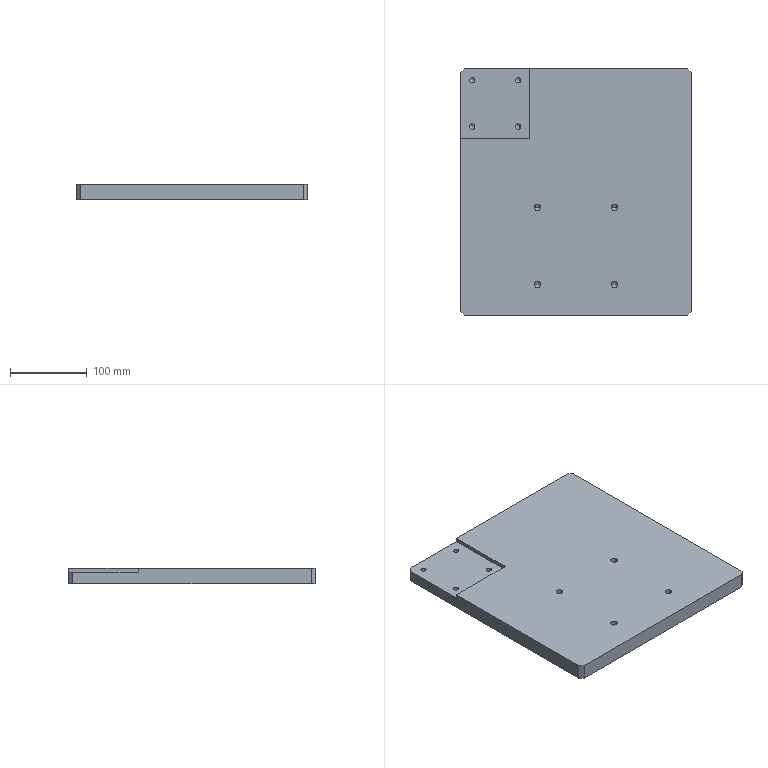Part | SolidWorks | features HoleWzd 2, Chamfer 1, Extrusion 1, ICE 1 | 1 solid | 45 faces | box 300 x 320 x 20 mm | volume 1873413 mm3 | cylinder 16 | cone 16 | plane 13 | commonest cylinder face diameters 6.8 x8 8.5 x8
STEP:
#1=CARTESIAN_POINT('',(-78.4,145.,-5.));
#2=VERTEX_POINT('',#1);
#3=CARTESIAN_POINT('',(-71.6,145.,-5.));
#4=VERTEX_POINT('',#3);
#5=CARTESIAN_POINT('',(-75.,145.,-5.));
#6=DIRECTION('',(0.,0.,1.));
#7=DIRECTION('',(1.,0.,0.));
#8=AXIS2_PLACEMENT_3D('',#5,#6,#7);
#9=CIRCLE('',#8,3.4);
#10=EDGE_CURVE('',#2,#4,#9,.T.);
#11=ORIENTED_EDGE('',*,*,#10,.F.);
#12=CARTESIAN_POINT('',(-78.4,145.,5.));
#13=VERTEX_POINT('',#12);
#14=CARTESIAN_POINT('',(-78.4,145.,5.));
#15=DIRECTION('',(0.,0.,1.));
#16=VECTOR('',#15,1000.);
#17=LINE('',#14,#16);
#18=EDGE_CURVE('',#2,#13,#17,.T.);
#19=ORIENTED_EDGE('',*,*,#18,.T.);
#20=CARTESIAN_POINT('',(-71.6,145.,5.));
#21=VERTEX_POINT('',#20);
#22=CARTESIAN_POINT('',(-75.,145.,5.));
#23=DIRECTION('',(0.,0.,1.));
#24=DIRECTION('',(1.,0.,0.));
#25=AXIS2_PLACEMENT_3D('',#22,#23,#24);
#26=CIRCLE('',#25,3.4);
#27=EDGE_CURVE('',#13,#21,#26,.T.);
#28=ORIENTED_EDGE('',*,*,#27,.T.);
#29=CARTESIAN_POINT('',(-71.6,145.,5.));
#30=DIRECTION('',(0.,0.,1.));
#31=VECTOR('',#30,1000.);
#32=LINE('',#29,#31);
#33=EDGE_CURVE('',#4,#21,#32,.T.);
#34=ORIENTED_EDGE('',*,*,#33,.F.);
#35=EDGE_LOOP('',(#11,#19,#28,#34));
#36=FACE_OUTER_BOUND('',#35,.T.);
#37=CARTESIAN_POINT('',(-75.,145.,5.));
#38=DIRECTION('',(0.,0.,1.));
#39=DIRECTION('',(1.,0.,0.));
#40=AXIS2_PLACEMENT_3D('',#37,#38,#39);
#41=CYLINDRICAL_SURFACE('',#40,3.4);
#42=ADVANCED_FACE('',(#36),#41,.F.);
#43=CARTESIAN_POINT('',(-75.,145.,-7.043));
#44=VERTEX_POINT('',#43);
#45=CARTESIAN_POINT('',(-71.6,145.,-5.));
#46=DIRECTION('',(0.8572,0.,0.515));
#47=VECTOR('',#46,1000.);
#48=LINE('',#45,#47);
#49=EDGE_CURVE('',#44,#4,#48,.T.);
#50=ORIENTED_EDGE('',*,*,#49,.F.);
#51=CARTESIAN_POINT('',(-78.4,145.,-5.));
#52=DIRECTION('',(-0.8572,0.,0.515));
#53=VECTOR('',#52,1000.);
#54=LINE('',#51,#53);
#55=EDGE_CURVE('',#44,#2,#54,.T.);
#56=ORIENTED_EDGE('',*,*,#55,.T.);
#57=ORIENTED_EDGE('',*,*,#10,.T.);
#58=EDGE_LOOP('',(#50,#56,#57));
#59=FACE_OUTER_BOUND('',#58,.T.);
#60=CARTESIAN_POINT('',(-75.,145.,-5.));
#61=DIRECTION('',(0.,0.,1.));
#62=DIRECTION('',(1.,0.,0.));
#63=AXIS2_PLACEMENT_3D('',#60,#61,#62);
#64=CONICAL_SURFACE('',#63,3.4,1.03);
#65=ADVANCED_FACE('',(#59),#64,.F.);
#66=CARTESIAN_POINT('',(-138.4,85.,-5.));
#67=VERTEX_POINT('',#66);
#68=CARTESIAN_POINT('',(-131.6,85.,-5.));
#69=VERTEX_POINT('',#68);
#70=CARTESIAN_POINT('',(-135.,85.,-5.));
#71=DIRECTION('',(0.,0.,1.));
#72=DIRECTION('',(1.,0.,0.));
#73=AXIS2_PLACEMENT_3D('',#70,#71,#72);
#74=CIRCLE('',#73,3.4);
#75=EDGE_CURVE('',#67,#69,#74,.T.);
#76=ORIENTED_EDGE('',*,*,#75,.F.);
#77=CARTESIAN_POINT('',(-138.4,85.,5.));
#78=VERTEX_POINT('',#77);
#79=CARTESIAN_POINT('',(-138.4,85.,5.));
#80=DIRECTION('',(0.,0.,1.));
#81=VECTOR('',#80,1000.);
#82=LINE('',#79,#81);
#83=EDGE_CURVE('',#67,#78,#82,.T.);
#84=ORIENTED_EDGE('',*,*,#83,.T.);
#85=CARTESIAN_POINT('',(-131.6,85.,5.));
#86=VERTEX_POINT('',#85);
#87=CARTESIAN_POINT('',(-135.,85.,5.));
#88=DIRECTION('',(0.,0.,1.));
#89=DIRECTION('',(1.,0.,0.));
#90=AXIS2_PLACEMENT_3D('',#87,#88,#89);
#91=CIRCLE('',#90,3.4);
#92=EDGE_CURVE('',#78,#86,#91,.T.);
#93=ORIENTED_EDGE('',*,*,#92,.T.);
#94=CARTESIAN_POINT('',(-131.6,85.,5.));
#95=DIRECTION('',(0.,0.,1.));
#96=VECTOR('',#95,1000.);
#97=LINE('',#94,#96);
#98=EDGE_CURVE('',#69,#86,#97,.T.);
#99=ORIENTED_EDGE('',*,*,#98,.F.);
#100=EDGE_LOOP('',(#76,#84,#93,#99));
#101=FACE_OUTER_BOUND('',#100,.T.);
#102=CARTESIAN_POINT('',(-135.,85.,5.));
#103=DIRECTION('',(0.,0.,1.));
#104=DIRECTION('',(1.,0.,0.));
#105=AXIS2_PLACEMENT_3D('',#102,#103,#104);
#106=CYLINDRICAL_SURFACE('',#105,3.4);
#107=ADVANCED_FACE('',(#101),#106,.F.);
#108=CARTESIAN_POINT('',(-135.,85.,-7.043));
#109=VERTEX_POINT('',#108);
#110=CARTESIAN_POINT('',(-131.6,85.,-5.));
#111=DIRECTION('',(0.8572,0.,0.515));
#112=VECTOR('',#111,1000.);
#113=LINE('',#110,#112);
#114=EDGE_CURVE('',#109,#69,#113,.T.);
#115=ORIENTED_EDGE('',*,*,#114,.F.);
#116=CARTESIAN_POINT('',(-138.4,85.,-5.));
#117=DIRECTION('',(-0.8572,0.,0.515));
#118=VECTOR('',#117,1000.);
#119=LINE('',#116,#118);
#120=EDGE_CURVE('',#109,#67,#119,.T.);
#121=ORIENTED_EDGE('',*,*,#120,.T.);
#122=ORIENTED_EDGE('',*,*,#75,.T.);
#123=EDGE_LOOP('',(#115,#121,#122));
#124=FACE_OUTER_BOUND('',#123,.T.);
#125=CARTESIAN_POINT('',(-135.,85.,-5.));
#126=DIRECTION('',(0.,0.,1.));
#127=DIRECTION('',(1.,0.,0.));
#128=AXIS2_PLACEMENT_3D('',#125,#126,#127);
#129=CONICAL_SURFACE('',#128,3.4,1.03);
#130=ADVANCED_FACE('',(#124),#129,.F.);
#131=CARTESIAN_POINT('',(-138.4,145.,-5.));
#132=VERTEX_POINT('',#131);
#133=CARTESIAN_POINT('',(-131.6,145.,-5.));
#134=VERTEX_POINT('',#133);
#135=CARTESIAN_POINT('',(-135.,145.,-5.));
#136=DIRECTION('',(0.,0.,1.));
#137=DIRECTION('',(1.,0.,0.));
#138=AXIS2_PLACEMENT_3D('',#135,#136,#137);
#139=CIRCLE('',#138,3.4);
#140=EDGE_CURVE('',#132,#134,#139,.T.);
#141=ORIENTED_EDGE('',*,*,#140,.F.);
#142=CARTESIAN_POINT('',(-138.4,145.,5.));
#143=VERTEX_POINT('',#142);
#144=CARTESIAN_POINT('',(-138.4,145.,5.));
#145=DIRECTION('',(0.,0.,1.));
#146=VECTOR('',#145,1000.);
#147=LINE('',#144,#146);
#148=EDGE_CURVE('',#132,#143,#147,.T.);
#149=ORIENTED_EDGE('',*,*,#148,.T.);
#150=CARTESIAN_POINT('',(-131.6,145.,5.));
#151=VERTEX_POINT('',#150);
#152=CARTESIAN_POINT('',(-135.,145.,5.));
#153=DIRECTION('',(0.,0.,1.));
#154=DIRECTION('',(1.,0.,0.));
#155=AXIS2_PLACEMENT_3D('',#152,#153,#154);
#156=CIRCLE('',#155,3.4);
#157=EDGE_CURVE('',#143,#151,#156,.T.);
#158=ORIENTED_EDGE('',*,*,#157,.T.);
#159=CARTESIAN_POINT('',(-131.6,145.,5.));
#160=DIRECTION('',(0.,0.,1.));
#161=VECTOR('',#160,1000.);
#162=LINE('',#159,#161);
#163=EDGE_CURVE('',#134,#151,#162,.T.);
#164=ORIENTED_EDGE('',*,*,#163,.F.);
#165=EDGE_LOOP('',(#141,#149,#158,#164));
#166=FACE_OUTER_BOUND('',#165,.T.);
#167=CARTESIAN_POINT('',(-135.,145.,5.));
#168=DIRECTION('',(0.,0.,1.));
#169=DIRECTION('',(1.,0.,0.));
#170=AXIS2_PLACEMENT_3D('',#167,#168,#169);
#171=CYLINDRICAL_SURFACE('',#170,3.4);
#172=ADVANCED_FACE('',(#166),#171,.F.);
#173=CARTESIAN_POINT('',(-135.,145.,-7.043));
#174=VERTEX_POINT('',#173);
#175=CARTESIAN_POINT('',(-131.6,145.,-5.));
#176=DIRECTION('',(0.8572,0.,0.515));
#177=VECTOR('',#176,1000.);
#178=LINE('',#175,#177);
#179=EDGE_CURVE('',#174,#134,#178,.T.);
#180=ORIENTED_EDGE('',*,*,#179,.F.);
#181=CARTESIAN_POINT('',(-138.4,145.,-5.));
#182=DIRECTION('',(-0.8572,0.,0.515));
#183=VECTOR('',#182,1000.);
#184=LINE('',#181,#183);
#185=EDGE_CURVE('',#174,#132,#184,.T.);
#186=ORIENTED_EDGE('',*,*,#185,.T.);
#187=ORIENTED_EDGE('',*,*,#140,.T.);
#188=EDGE_LOOP('',(#180,#186,#187));
#189=FACE_OUTER_BOUND('',#188,.T.);
#190=CARTESIAN_POINT('',(-135.,145.,-5.));
#191=DIRECTION('',(0.,0.,1.));
#192=DIRECTION('',(1.,0.,0.));
#193=AXIS2_PLACEMENT_3D('',#190,#191,#192);
#194=CONICAL_SURFACE('',#193,3.4,1.03);
#195=ADVANCED_FACE('',(#189),#194,.F.);
#196=CARTESIAN_POINT('',(-78.4,85.,-5.));
#197=VERTEX_POINT('',#196);
#198=CARTESIAN_POINT('',(-71.6,85.,-5.));
#199=VERTEX_POINT('',#198);
#200=CARTESIAN_POINT('',(-75.,85.,-5.));
#201=DIRECTION('',(0.,0.,1.));
#202=DIRECTION('',(1.,0.,0.));
#203=AXIS2_PLACEMENT_3D('',#200,#201,#202);
#204=CIRCLE('',#203,3.4);
#205=EDGE_CURVE('',#197,#199,#204,.T.);
#206=ORIENTED_EDGE('',*,*,#205,.F.);
#207=CARTESIAN_POINT('',(-78.4,85.,5.));
#208=VERTEX_POINT('',#207);
#209=CARTESIAN_POINT('',(-78.4,85.,5.));
#210=DIRECTION('',(0.,0.,1.));
#211=VECTOR('',#210,1000.);
#212=LINE('',#209,#211);
#213=EDGE_CURVE('',#197,#208,#212,.T.);
#214=ORIENTED_EDGE('',*,*,#213,.T.);
#215=CARTESIAN_POINT('',(-71.6,85.,5.));
#216=VERTEX_POINT('',#215);
#217=CARTESIAN_POINT('',(-75.,85.,5.));
#218=DIRECTION('',(0.,0.,1.));
#219=DIRECTION('',(1.,0.,0.));
#220=AXIS2_PLACEMENT_3D('',#217,#218,#219);
#221=CIRCLE('',#220,3.4);
#222=EDGE_CURVE('',#208,#216,#221,.T.);
#223=ORIENTED_EDGE('',*,*,#222,.T.);
#224=CARTESIAN_POINT('',(-71.6,85.,5.));
#225=DIRECTION('',(0.,0.,1.));
#226=VECTOR('',#225,1000.);
#227=LINE('',#224,#226);
#228=EDGE_CURVE('',#199,#216,#227,.T.);
#229=ORIENTED_EDGE('',*,*,#228,.F.);
#230=EDGE_LOOP('',(#206,#214,#223,#229));
#231=FACE_OUTER_BOUND('',#230,.T.);
#232=CARTESIAN_POINT('',(-75.,85.,5.));
#233=DIRECTION('',(0.,0.,1.));
#234=DIRECTION('',(1.,0.,0.));
#235=AXIS2_PLACEMENT_3D('',#232,#233,#234);
#236=CYLINDRICAL_SURFACE('',#235,3.4);
#237=ADVANCED_FACE('',(#231),#236,.F.);
#238=CARTESIAN_POINT('',(-75.,85.,-7.043));
#239=VERTEX_POINT('',#238);
#240=CARTESIAN_POINT('',(-71.6,85.,-5.));
#241=DIRECTION('',(0.8572,0.,0.515));
#242=VECTOR('',#241,1000.);
#243=LINE('',#240,#242);
#244=EDGE_CURVE('',#239,#199,#243,.T.);
#245=ORIENTED_EDGE('',*,*,#244,.F.);
#246=CARTESIAN_POINT('',(-78.4,85.,-5.));
#247=DIRECTION('',(-0.8572,0.,0.515));
#248=VECTOR('',#247,1000.);
#249=LINE('',#246,#248);
#250=EDGE_CURVE('',#239,#197,#249,.T.);
#251=ORIENTED_EDGE('',*,*,#250,.T.);
#252=ORIENTED_EDGE('',*,*,#205,.T.);
#253=EDGE_LOOP('',(#245,#251,#252));
#254=FACE_OUTER_BOUND('',#253,.T.);
#255=CARTESIAN_POINT('',(-75.,85.,-5.));
#256=DIRECTION('',(0.,0.,1.));
#257=DIRECTION('',(1.,0.,0.));
#258=AXIS2_PLACEMENT_3D('',#255,#256,#257);
#259=CONICAL_SURFACE('',#258,3.4,1.03);
#260=ADVANCED_FACE('',(#254),#259,.F.);
#261=CARTESIAN_POINT('',(45.75,-20.,-5.));
#262=VERTEX_POINT('',#261);
#263=CARTESIAN_POINT('',(54.25,-20.,-5.));
#264=VERTEX_POINT('',#263);
#265=CARTESIAN_POINT('',(50.,-20.,-5.));
#266=DIRECTION('',(0.,0.,1.));
#267=DIRECTION('',(1.,0.,0.));
#268=AXIS2_PLACEMENT_3D('',#265,#266,#267);
#269=CIRCLE('',#268,4.25);
#270=EDGE_CURVE('',#262,#264,#269,.T.);
#271=ORIENTED_EDGE('',*,*,#270,.F.);
#272=CARTESIAN_POINT('',(45.75,-20.,10.));
#273=VERTEX_POINT('',#272);
#274=CARTESIAN_POINT('',(45.75,-20.,10.));
#275=DIRECTION('',(0.,0.,1.));
#276=VECTOR('',#275,1000.);
#277=LINE('',#274,#276);
#278=EDGE_CURVE('',#262,#273,#277,.T.);
#279=ORIENTED_EDGE('',*,*,#278,.T.);
#280=CARTESIAN_POINT('',(54.25,-20.,10.));
#281=VERTEX_POINT('',#280);
#282=CARTESIAN_POINT('',(50.,-20.,10.));
#283=DIRECTION('',(0.,0.,1.));
#284=DIRECTION('',(1.,0.,0.));
#285=AXIS2_PLACEMENT_3D('',#282,#283,#284);
#286=CIRCLE('',#285,4.25);
#287=EDGE_CURVE('',#273,#281,#286,.T.);
#288=ORIENTED_EDGE('',*,*,#287,.T.);
#289=CARTESIAN_POINT('',(54.25,-20.,10.));
#290=DIRECTION('',(0.,0.,1.));
#291=VECTOR('',#290,1000.);
#292=LINE('',#289,#291);
#293=EDGE_CURVE('',#264,#281,#292,.T.);
#294=ORIENTED_EDGE('',*,*,#293,.F.);
#295=EDGE_LOOP('',(#271,#279,#288,#294));
#296=FACE_OUTER_BOUND('',#295,.T.);
#297=CARTESIAN_POINT('',(50.,-20.,10.));
#298=DIRECTION('',(0.,0.,1.));
#299=DIRECTION('',(1.,0.,0.));
#300=AXIS2_PLACEMENT_3D('',#297,#298,#299);
#301=CYLINDRICAL_SURFACE('',#300,4.25);
#302=ADVANCED_FACE('',(#296),#301,.F.);
#303=CARTESIAN_POINT('',(50.,-20.,-7.554));
#304=VERTEX_POINT('',#303);
#305=CARTESIAN_POINT('',(54.25,-20.,-5.));
#306=DIRECTION('',(0.8572,0.,0.515));
#307=VECTOR('',#306,1000.);
#308=LINE('',#305,#307);
#309=EDGE_CURVE('',#304,#264,#308,.T.);
#310=ORIENTED_EDGE('',*,*,#309,.F.);
#311=CARTESIAN_POINT('',(45.75,-20.,-5.));
#312=DIRECTION('',(-0.8572,0.,0.515));
#313=VECTOR('',#312,1000.);
#314=LINE('',#311,#313);
#315=EDGE_CURVE('',#304,#262,#314,.T.);
#316=ORIENTED_EDGE('',*,*,#315,.T.);
#317=ORIENTED_EDGE('',*,*,#270,.T.);
#318=EDGE_LOOP('',(#310,#316,#317));
#319=FACE_OUTER_BOUND('',#318,.T.);
#320=CARTESIAN_POINT('',(50.,-20.,-5.));
#321=DIRECTION('',(0.,0.,1.));
#322=DIRECTION('',(1.,0.,0.));
#323=AXIS2_PLACEMENT_3D('',#320,#321,#322);
#324=CONICAL_SURFACE('',#323,4.25,1.03);
#325=ADVANCED_FACE('',(#319),#324,.F.);
#326=CARTESIAN_POINT('',(-54.25,-120.,-5.));
#327=VERTEX_POINT('',#326);
#328=CARTESIAN_POINT('',(-45.75,-120.,-5.));
#329=VERTEX_POINT('',#328);
#330=CARTESIAN_POINT('',(-50.,-120.,-5.));
#331=DIRECTION('',(0.,0.,1.));
#332=DIRECTION('',(1.,0.,0.));
#333=AXIS2_PLACEMENT_3D('',#330,#331,#332);
#334=CIRCLE('',#333,4.25);
#335=EDGE_CURVE('',#327,#329,#334,.T.);
#336=ORIENTED_EDGE('',*,*,#335,.F.);
#337=CARTESIAN_POINT('',(-54.25,-120.,10.));
#338=VERTEX_POINT('',#337);
#339=CARTESIAN_POINT('',(-54.25,-120.,10.));
#340=DIRECTION('',(0.,0.,1.));
#341=VECTOR('',#340,1000.);
#342=LINE('',#339,#341);
#343=EDGE_CURVE('',#327,#338,#342,.T.);
#344=ORIENTED_EDGE('',*,*,#343,.T.);
#345=CARTESIAN_POINT('',(-45.75,-120.,10.));
#346=VERTEX_POINT('',#345);
#347=CARTESIAN_POINT('',(-50.,-120.,10.));
#348=DIRECTION('',(0.,0.,1.));
#349=DIRECTION('',(1.,0.,0.));
#350=AXIS2_PLACEMENT_3D('',#347,#348,#349);
#351=CIRCLE('',#350,4.25);
#352=EDGE_CURVE('',#338,#346,#351,.T.);
#353=ORIENTED_EDGE('',*,*,#352,.T.);
#354=CARTESIAN_POINT('',(-45.75,-120.,10.));
#355=DIRECTION('',(0.,0.,1.));
#356=VECTOR('',#355,1000.);
#357=LINE('',#354,#356);
#358=EDGE_CURVE('',#329,#346,#357,.T.);
#359=ORIENTED_EDGE('',*,*,#358,.F.);
#360=EDGE_LOOP('',(#336,#344,#353,#359));
#361=FACE_OUTER_BOUND('',#360,.T.);
#362=CARTESIAN_POINT('',(-50.,-120.,10.));
#363=DIRECTION('',(0.,0.,1.));
#364=DIRECTION('',(1.,0.,0.));
#365=AXIS2_PLACEMENT_3D('',#362,#363,#364);
#366=CYLINDRICAL_SURFACE('',#365,4.25);
#367=ADVANCED_FACE('',(#361),#366,.F.);
#368=CARTESIAN_POINT('',(-50.,-120.,-7.554));
#369=VERTEX_POINT('',#368);
#370=CARTESIAN_POINT('',(-45.75,-120.,-5.));
#371=DIRECTION('',(0.8572,0.,0.515));
#372=VECTOR('',#371,1000.);
#373=LINE('',#370,#372);
#374=EDGE_CURVE('',#369,#329,#373,.T.);
#375=ORIENTED_EDGE('',*,*,#374,.F.);
#376=CARTESIAN_POINT('',(-54.25,-120.,-5.));
#377=DIRECTION('',(-0.8572,0.,0.515));
#378=VECTOR('',#377,1000.);
#379=LINE('',#376,#378);
#380=EDGE_CURVE('',#369,#327,#379,.T.);
#381=ORIENTED_EDGE('',*,*,#380,.T.);
#382=ORIENTED_EDGE('',*,*,#335,.T.);
#383=EDGE_LOOP('',(#375,#381,#382));
#384=FACE_OUTER_BOUND('',#383,.T.);
#385=CARTESIAN_POINT('',(-50.,-120.,-5.));
#386=DIRECTION('',(0.,0.,1.));
#387=DIRECTION('',(1.,0.,0.));
#388=AXIS2_PLACEMENT_3D('',#385,#386,#387);
#389=CONICAL_SURFACE('',#388,4.25,1.03);
#390=ADVANCED_FACE('',(#384),#389,.F.);
#391=CARTESIAN_POINT('',(-54.25,-20.,-5.));
#392=VERTEX_POINT('',#391);
#393=CARTESIAN_POINT('',(-45.75,-20.,-5.));
#394=VERTEX_POINT('',#393);
#395=CARTESIAN_POINT('',(-50.,-20.,-5.));
#396=DIRECTION('',(0.,0.,1.));
#397=DIRECTION('',(1.,0.,0.));
#398=AXIS2_PLACEMENT_3D('',#395,#396,#397);
#399=CIRCLE('',#398,4.25);
#400=EDGE_CURVE('',#392,#394,#399,.T.);
#401=ORIENTED_EDGE('',*,*,#400,.F.);
#402=CARTESIAN_POINT('',(-54.25,-20.,10.));
#403=VERTEX_POINT('',#402);
#404=CARTESIAN_POINT('',(-54.25,-20.,10.));
#405=DIRECTION('',(0.,0.,1.));
#406=VECTOR('',#405,1000.);
#407=LINE('',#404,#406);
#408=EDGE_CURVE('',#392,#403,#407,.T.);
#409=ORIENTED_EDGE('',*,*,#408,.T.);
#410=CARTESIAN_POINT('',(-45.75,-20.,10.));
#411=VERTEX_POINT('',#410);
#412=CARTESIAN_POINT('',(-50.,-20.,10.));
#413=DIRECTION('',(0.,0.,1.));
#414=DIRECTION('',(1.,0.,0.));
#415=AXIS2_PLACEMENT_3D('',#412,#413,#414);
#416=CIRCLE('',#415,4.25);
#417=EDGE_CURVE('',#403,#411,#416,.T.);
#418=ORIENTED_EDGE('',*,*,#417,.T.);
#419=CARTESIAN_POINT('',(-45.75,-20.,10.));
#420=DIRECTION('',(0.,0.,1.));
#421=VECTOR('',#420,1000.);
#422=LINE('',#419,#421);
#423=EDGE_CURVE('',#394,#411,#422,.T.);
#424=ORIENTED_EDGE('',*,*,#423,.F.);
#425=EDGE_LOOP('',(#401,#409,#418,#424));
#426=FACE_OUTER_BOUND('',#425,.T.);
#427=CARTESIAN_POINT('',(-50.,-20.,10.));
#428=DIRECTION('',(0.,0.,1.));
#429=DIRECTION('',(1.,0.,0.));
#430=AXIS2_PLACEMENT_3D('',#427,#428,#429);
#431=CYLINDRICAL_SURFACE('',#430,4.25);
#432=ADVANCED_FACE('',(#426),#431,.F.);
#433=CARTESIAN_POINT('',(-50.,-20.,-7.554));
#434=VERTEX_POINT('',#433);
#435=CARTESIAN_POINT('',(-45.75,-20.,-5.));
#436=DIRECTION('',(0.8572,0.,0.515));
#437=VECTOR('',#436,1000.);
#438=LINE('',#435,#437);
#439=EDGE_CURVE('',#434,#394,#438,.T.);
#440=ORIENTED_EDGE('',*,*,#439,.F.);
#441=CARTESIAN_POINT('',(-54.25,-20.,-5.));
#442=DIRECTION('',(-0.8572,0.,0.515));
#443=VECTOR('',#442,1000.);
#444=LINE('',#441,#443);
#445=EDGE_CURVE('',#434,#392,#444,.T.);
#446=ORIENTED_EDGE('',*,*,#445,.T.);
#447=ORIENTED_EDGE('',*,*,#400,.T.);
#448=EDGE_LOOP('',(#440,#446,#447));
#449=FACE_OUTER_BOUND('',#448,.T.);
#450=CARTESIAN_POINT('',(-50.,-20.,-5.));
#451=DIRECTION('',(0.,0.,1.));
#452=DIRECTION('',(1.,0.,0.));
#453=AXIS2_PLACEMENT_3D('',#450,#451,#452);
#454=CONICAL_SURFACE('',#453,4.25,1.03);
#455=ADVANCED_FACE('',(#449),#454,.F.);
#456=CARTESIAN_POINT('',(45.75,-120.,-5.));
#457=VERTEX_POINT('',#456);
#458=CARTESIAN_POINT('',(54.25,-120.,-5.));
#459=VERTEX_POINT('',#458);
#460=CARTESIAN_POINT('',(50.,-120.,-5.));
#461=DIRECTION('',(0.,0.,1.));
#462=DIRECTION('',(1.,0.,0.));
#463=AXIS2_PLACEMENT_3D('',#460,#461,#462);
#464=CIRCLE('',#463,4.25);
#465=EDGE_CURVE('',#457,#459,#464,.T.);
#466=ORIENTED_EDGE('',*,*,#465,.F.);
#467=CARTESIAN_POINT('',(45.75,-120.,10.));
#468=VERTEX_POINT('',#467);
#469=CARTESIAN_POINT('',(45.75,-120.,10.));
#470=DIRECTION('',(0.,0.,1.));
#471=VECTOR('',#470,1000.);
#472=LINE('',#469,#471);
#473=EDGE_CURVE('',#457,#468,#472,.T.);
#474=ORIENTED_EDGE('',*,*,#473,.T.);
#475=CARTESIAN_POINT('',(54.25,-120.,10.));
#476=VERTEX_POINT('',#475);
#477=CARTESIAN_POINT('',(50.,-120.,10.));
#478=DIRECTION('',(0.,0.,1.));
#479=DIRECTION('',(1.,0.,0.));
#480=AXIS2_PLACEMENT_3D('',#477,#478,#479);
#481=CIRCLE('',#480,4.25);
#482=EDGE_CURVE('',#468,#476,#481,.T.);
#483=ORIENTED_EDGE('',*,*,#482,.T.);
#484=CARTESIAN_POINT('',(54.25,-120.,10.));
#485=DIRECTION('',(0.,0.,1.));
#486=VECTOR('',#485,1000.);
#487=LINE('',#484,#486);
#488=EDGE_CURVE('',#459,#476,#487,.T.);
#489=ORIENTED_EDGE('',*,*,#488,.F.);
#490=EDGE_LOOP('',(#466,#474,#483,#489));
#491=FACE_OUTER_BOUND('',#490,.T.);
#492=CARTESIAN_POINT('',(50.,-120.,10.));
#493=DIRECTION('',(0.,0.,1.));
#494=DIRECTION('',(1.,0.,0.));
#495=AXIS2_PLACEMENT_3D('',#492,#493,#494);
#496=CYLINDRICAL_SURFACE('',#495,4.25);
#497=ADVANCED_FACE('',(#491),#496,.F.);
#498=CARTESIAN_POINT('',(50.,-120.,-7.554));
#499=VERTEX_POINT('',#498);
#500=CARTESIAN_POINT('',(54.25,-120.,-5.));
#501=DIRECTION('',(0.8572,0.,0.515));
#502=VECTOR('',#501,1000.);
#503=LINE('',#500,#502);
#504=EDGE_CURVE('',#499,#459,#503,.T.);
#505=ORIENTED_EDGE('',*,*,#504,.F.);
#506=CARTESIAN_POINT('',(45.75,-120.,-5.));
#507=DIRECTION('',(-0.8572,0.,0.515));
#508=VECTOR('',#507,1000.);
#509=LINE('',#506,#508);
#510=EDGE_CURVE('',#499,#457,#509,.T.);
#511=ORIENTED_EDGE('',*,*,#510,.T.);
#512=ORIENTED_EDGE('',*,*,#465,.T.);
#513=EDGE_LOOP('',(#505,#511,#512));
#514=FACE_OUTER_BOUND('',#513,.T.);
#515=CARTESIAN_POINT('',(50.,-120.,-5.));
#516=DIRECTION('',(0.,0.,1.));
#517=DIRECTION('',(1.,0.,0.));
#518=AXIS2_PLACEMENT_3D('',#515,#516,#517);
#519=CONICAL_SURFACE('',#518,4.25,1.03);
#520=ADVANCED_FACE('',(#514),#519,.F.);
#521=CARTESIAN_POINT('',(150.,-155.,10.));
#522=VERTEX_POINT('',#521);
#523=CARTESIAN_POINT('',(150.,155.,10.));
#524=VERTEX_POINT('',#523);
#525=CARTESIAN_POINT('',(150.,-160.,10.));
#526=DIRECTION('',(0.,1.,0.));
#527=VECTOR('',#526,1000.);
#528=LINE('',#525,#527);
#529=EDGE_CURVE('',#522,#524,#528,.T.);
#530=ORIENTED_EDGE('',*,*,#529,.F.);
#531=CARTESIAN_POINT('',(150.,-155.,-10.));
#532=VERTEX_POINT('',#531);
#533=CARTESIAN_POINT('',(150.,-155.,10.));
#534=DIRECTION('',(0.,0.,-1.));
#535=VECTOR('',#534,1000.);
#536=LINE('',#533,#535);
#537=EDGE_CURVE('',#522,#532,#536,.T.);
#538=ORIENTED_EDGE('',*,*,#537,.T.);
#539=CARTESIAN_POINT('',(150.,155.,-10.));
#540=VERTEX_POINT('',#539);
#541=CARTESIAN_POINT('',(150.,-160.,-10.));
#542=DIRECTION('',(0.,1.,0.));
#543=VECTOR('',#542,1000.);
#544=LINE('',#541,#543);
#545=EDGE_CURVE('',#532,#540,#544,.T.);
#546=ORIENTED_EDGE('',*,*,#545,.T.);
#547=CARTESIAN_POINT('',(150.,155.,10.));
#548=DIRECTION('',(0.,0.,1.));
#549=VECTOR('',#548,1000.);
#550=LINE('',#547,#549);
#551=EDGE_CURVE('',#540,#524,#550,.T.);
#552=ORIENTED_EDGE('',*,*,#551,.T.);
#553=EDGE_LOOP('',(#530,#538,#546,#552));
#554=FACE_OUTER_BOUND('',#553,.T.);
#555=CARTESIAN_POINT('',(150.,-160.,10.));
#556=DIRECTION('',(-1.,0.,0.));
#557=DIRECTION('',(0.,0.,1.));
#558=AXIS2_PLACEMENT_3D('',#555,#556,#557);
#559=PLANE('',#558);
#560=ADVANCED_FACE('',(#554),#559,.F.);
#561=CARTESIAN_POINT('',(145.,160.,10.));
#562=VERTEX_POINT('',#561);
#563=CARTESIAN_POINT('',(-60.,160.,10.));
#564=VERTEX_POINT('',#563);
#565=CARTESIAN_POINT('',(-150.,160.,10.));
#566=DIRECTION('',(-1.,0.,0.));
#567=VECTOR('',#566,1000.);
#568=LINE('',#565,#567);
#569=EDGE_CURVE('',#562,#564,#568,.T.);
#570=ORIENTED_EDGE('',*,*,#569,.F.);
#571=CARTESIAN_POINT('',(145.,160.,-10.));
#572=VERTEX_POINT('',#571);
#573=CARTESIAN_POINT('',(145.,160.,10.));
#574=DIRECTION('',(0.,0.,-1.));
#575=VECTOR('',#574,1000.);
#576=LINE('',#573,#575);
#577=EDGE_CURVE('',#562,#572,#576,.T.);
#578=ORIENTED_EDGE('',*,*,#577,.T.);
#579=CARTESIAN_POINT('',(-145.,160.,-10.));
#580=VERTEX_POINT('',#579);
#581=CARTESIAN_POINT('',(-150.,160.,-10.));
#582=DIRECTION('',(-1.,0.,0.));
#583=VECTOR('',#582,1000.);
#584=LINE('',#581,#583);
#585=EDGE_CURVE('',#572,#580,#584,.T.);
#586=ORIENTED_EDGE('',*,*,#585,.T.);
#587=CARTESIAN_POINT('',(-145.,160.,5.));
#588=VERTEX_POINT('',#587);
#589=CARTESIAN_POINT('',(-145.,160.,10.));
#590=DIRECTION('',(0.,0.,1.));
#591=VECTOR('',#590,1000.);
#592=LINE('',#589,#591);
#593=EDGE_CURVE('',#580,#588,#592,.T.);
#594=ORIENTED_EDGE('',*,*,#593,.T.);
#595=CARTESIAN_POINT('',(-60.,160.,5.));
#596=VERTEX_POINT('',#595);
#597=CARTESIAN_POINT('',(-150.,160.,5.));
#598=DIRECTION('',(-1.,0.,0.));
#599=VECTOR('',#598,1000.);
#600=LINE('',#597,#599);
#601=EDGE_CURVE('',#596,#588,#600,.T.);
#602=ORIENTED_EDGE('',*,*,#601,.F.);
#603=CARTESIAN_POINT('',(-60.,160.,5.));
#604=DIRECTION('',(0.,0.,1.));
#605=VECTOR('',#604,1000.);
#606=LINE('',#603,#605);
#607=EDGE_CURVE('',#596,#564,#606,.T.);
#608=ORIENTED_EDGE('',*,*,#607,.T.);
#609=EDGE_LOOP('',(#570,#578,#586,#594,#602,#608));
#610=FACE_OUTER_BOUND('',#609,.T.);
#611=CARTESIAN_POINT('',(-150.,160.,10.));
#612=DIRECTION('',(0.,-1.,0.));
#613=DIRECTION('',(0.,0.,-1.));
#614=AXIS2_PLACEMENT_3D('',#611,#612,#613);
#615=PLANE('',#614);
#616=ADVANCED_FACE('',(#610),#615,.F.);
#617=CARTESIAN_POINT('',(-150.,155.,-10.));
#618=VERTEX_POINT('',#617);
#619=CARTESIAN_POINT('',(-150.,-155.,-10.));
#620=VERTEX_POINT('',#619);
#621=CARTESIAN_POINT('',(-150.,-160.,-10.));
#622=DIRECTION('',(0.,-1.,0.));
#623=VECTOR('',#622,1000.);
#624=LINE('',#621,#623);
#625=EDGE_CURVE('',#618,#620,#624,.T.);
#626=ORIENTED_EDGE('',*,*,#625,.T.);
#627=CARTESIAN_POINT('',(-150.,-155.,10.));
#628=VERTEX_POINT('',#627);
#629=CARTESIAN_POINT('',(-150.,-155.,10.));
#630=DIRECTION('',(0.,0.,1.));
#631=VECTOR('',#630,1000.);
#632=LINE('',#629,#631);
#633=EDGE_CURVE('',#620,#628,#632,.T.);
#634=ORIENTED_EDGE('',*,*,#633,.T.);
#635=CARTESIAN_POINT('',(-150.,70.,10.));
#636=VERTEX_POINT('',#635);
#637=CARTESIAN_POINT('',(-150.,-160.,10.));
#638=DIRECTION('',(0.,-1.,0.));
#639=VECTOR('',#638,1000.);
#640=LINE('',#637,#639);
#641=EDGE_CURVE('',#636,#628,#640,.T.);
#642=ORIENTED_EDGE('',*,*,#641,.F.);
#643=CARTESIAN_POINT('',(-150.,70.,5.));
#644=VERTEX_POINT('',#643);
#645=CARTESIAN_POINT('',(-150.,70.,5.));
#646=DIRECTION('',(0.,0.,1.));
#647=VECTOR('',#646,1000.);
#648=LINE('',#645,#647);
#649=EDGE_CURVE('',#644,#636,#648,.T.);
#650=ORIENTED_EDGE('',*,*,#649,.F.);
#651=CARTESIAN_POINT('',(-150.,155.,5.));
#652=VERTEX_POINT('',#651);
#653=CARTESIAN_POINT('',(-150.,160.,5.));
#654=DIRECTION('',(0.,-1.,0.));
#655=VECTOR('',#654,1000.);
#656=LINE('',#653,#655);
#657=EDGE_CURVE('',#652,#644,#656,.T.);
#658=ORIENTED_EDGE('',*,*,#657,.F.);
#659=CARTESIAN_POINT('',(-150.,155.,10.));
#660=DIRECTION('',(0.,0.,-1.));
#661=VECTOR('',#660,1000.);
#662=LINE('',#659,#661);
#663=EDGE_CURVE('',#652,#618,#662,.T.);
#664=ORIENTED_EDGE('',*,*,#663,.T.);
#665=EDGE_LOOP('',(#626,#634,#642,#650,#658,#664));
#666=FACE_OUTER_BOUND('',#665,.T.);
#667=CARTESIAN_POINT('',(-150.,-160.,10.));
#668=DIRECTION('',(1.,0.,0.));
#669=DIRECTION('',(0.,0.,-1.));
#670=AXIS2_PLACEMENT_3D('',#667,#668,#669);
#671=PLANE('',#670);
#672=ADVANCED_FACE('',(#666),#671,.F.);
#673=CARTESIAN_POINT('',(-145.,-160.,10.));
#674=VERTEX_POINT('',#673);
#675=CARTESIAN_POINT('',(145.,-160.,10.));
#676=VERTEX_POINT('',#675);
#677=CARTESIAN_POINT('',(-150.,-160.,10.));
#678=DIRECTION('',(1.,0.,0.));
#679=VECTOR('',#678,1000.);
#680=LINE('',#677,#679);
#681=EDGE_CURVE('',#674,#676,#680,.T.);
#682=ORIENTED_EDGE('',*,*,#681,.F.);
#683=CARTESIAN_POINT('',(-145.,-160.,-10.));
#684=VERTEX_POINT('',#683);
#685=CARTESIAN_POINT('',(-145.,-160.,10.));
#686=DIRECTION('',(0.,0.,-1.));
#687=VECTOR('',#686,1000.);
#688=LINE('',#685,#687);
#689=EDGE_CURVE('',#674,#684,#688,.T.);
#690=ORIENTED_EDGE('',*,*,#689,.T.);
#691=CARTESIAN_POINT('',(145.,-160.,-10.));
#692=VERTEX_POINT('',#691);
#693=CARTESIAN_POINT('',(-150.,-160.,-10.));
#694=DIRECTION('',(1.,0.,0.));
#695=VECTOR('',#694,1000.);
#696=LINE('',#693,#695);
#697=EDGE_CURVE('',#684,#692,#696,.T.);
#698=ORIENTED_EDGE('',*,*,#697,.T.);
#699=CARTESIAN_POINT('',(145.,-160.,10.));
#700=DIRECTION('',(0.,0.,1.));
#701=VECTOR('',#700,1000.);
#702=LINE('',#699,#701);
#703=EDGE_CURVE('',#692,#676,#702,.T.);
#704=ORIENTED_EDGE('',*,*,#703,.T.);
#705=EDGE_LOOP('',(#682,#690,#698,#704));
#706=FACE_OUTER_BOUND('',#705,.T.);
#707=CARTESIAN_POINT('',(-150.,-160.,10.));
#708=DIRECTION('',(0.,1.,0.));
#709=DIRECTION('',(0.,0.,1.));
#710=AXIS2_PLACEMENT_3D('',#707,#708,#709);
#711=PLANE('',#710);
#712=ADVANCED_FACE('',(#706),#711,.F.);
#713=CARTESIAN_POINT('',(50.,-20.,10.));
#714=DIRECTION('',(0.,0.,1.));
#715=DIRECTION('',(1.,0.,0.));
#716=AXIS2_PLACEMENT_3D('',#713,#714,#715);
#717=CIRCLE('',#716,4.25);
#718=EDGE_CURVE('',#281,#273,#717,.T.);
#719=ORIENTED_EDGE('',*,*,#718,.F.);
#720=ORIENTED_EDGE('',*,*,#287,.F.);
#721=EDGE_LOOP('',(#719,#720));
#722=FACE_BOUND('',#721,.T.);
#723=CARTESIAN_POINT('',(-50.,-120.,10.));
#724=DIRECTION('',(0.,0.,1.));
#725=DIRECTION('',(1.,0.,0.));
#726=AXIS2_PLACEMENT_3D('',#723,#724,#725);
#727=CIRCLE('',#726,4.25);
#728=EDGE_CURVE('',#346,#338,#727,.T.);
#729=ORIENTED_EDGE('',*,*,#728,.F.);
#730=ORIENTED_EDGE('',*,*,#352,.F.);
#731=EDGE_LOOP('',(#729,#730));
#732=FACE_BOUND('',#731,.T.);
#733=CARTESIAN_POINT('',(-50.,-20.,10.));
#734=DIRECTION('',(0.,0.,1.));
#735=DIRECTION('',(1.,0.,0.));
#736=AXIS2_PLACEMENT_3D('',#733,#734,#735);
#737=CIRCLE('',#736,4.25);
#738=EDGE_CURVE('',#411,#403,#737,.T.);
#739=ORIENTED_EDGE('',*,*,#738,.F.);
#740=ORIENTED_EDGE('',*,*,#417,.F.);
#741=EDGE_LOOP('',(#739,#740));
#742=FACE_BOUND('',#741,.T.);
#743=CARTESIAN_POINT('',(50.,-120.,10.));
#744=DIRECTION('',(0.,0.,1.));
#745=DIRECTION('',(1.,0.,0.));
#746=AXIS2_PLACEMENT_3D('',#743,#744,#745);
#747=CIRCLE('',#746,4.25);
#748=EDGE_CURVE('',#476,#468,#747,.T.);
#749=ORIENTED_EDGE('',*,*,#748,.F.);
#750=ORIENTED_EDGE('',*,*,#482,.F.);
#751=EDGE_LOOP('',(#749,#750));
#752=FACE_BOUND('',#751,.T.);
#753=ORIENTED_EDGE('',*,*,#641,.T.);
#754=CARTESIAN_POINT('',(-145.,-160.,10.));
#755=DIRECTION('',(0.7071,-0.7071,0.));
#756=VECTOR('',#755,1000.);
#757=LINE('',#754,#756);
#758=EDGE_CURVE('',#628,#674,#757,.T.);
#759=ORIENTED_EDGE('',*,*,#758,.T.);
#760=ORIENTED_EDGE('',*,*,#681,.T.);
#761=CARTESIAN_POINT('',(150.,-155.,10.));
#762=DIRECTION('',(0.7071,0.7071,0.));
#763=VECTOR('',#762,1000.);
#764=LINE('',#761,#763);
#765=EDGE_CURVE('',#676,#522,#764,.T.);
#766=ORIENTED_EDGE('',*,*,#765,.T.);
#767=ORIENTED_EDGE('',*,*,#529,.T.);
#768=CARTESIAN_POINT('',(145.,160.,10.));
#769=DIRECTION('',(-0.7071,0.7071,0.));
#770=VECTOR('',#769,1000.);
#771=LINE('',#768,#770);
#772=EDGE_CURVE('',#524,#562,#771,.T.);
#773=ORIENTED_EDGE('',*,*,#772,.T.);
#774=ORIENTED_EDGE('',*,*,#569,.T.);
#775=CARTESIAN_POINT('',(-60.,70.,10.));
#776=VERTEX_POINT('',#775);
#777=CARTESIAN_POINT('',(-60.,160.,10.));
#778=DIRECTION('',(0.,1.,0.));
#779=VECTOR('',#778,1000.);
#780=LINE('',#777,#779);
#781=EDGE_CURVE('',#776,#564,#780,.T.);
#782=ORIENTED_EDGE('',*,*,#781,.F.);
#783=CARTESIAN_POINT('',(-150.,70.,10.));
#784=DIRECTION('',(1.,0.,0.));
#785=VECTOR('',#784,1000.);
#786=LINE('',#783,#785);
#787=EDGE_CURVE('',#636,#776,#786,.T.);
#788=ORIENTED_EDGE('',*,*,#787,.F.);
#789=EDGE_LOOP('',(#753,#759,#760,#766,#767,#773,#774,#782,#788));
#790=FACE_OUTER_BOUND('',#789,.T.);
#791=CARTESIAN_POINT('',(0.,0.,10.));
#792=DIRECTION('',(0.,0.,-1.));
#793=DIRECTION('',(-1.,0.,0.));
#794=AXIS2_PLACEMENT_3D('',#791,#792,#793);
#795=PLANE('',#794);
#796=ADVANCED_FACE('',(#722,#732,#742,#752,#790),#795,.F.);
#797=ORIENTED_EDGE('',*,*,#697,.F.);
#798=CARTESIAN_POINT('',(-152.5,-152.5,-10.));
#799=DIRECTION('',(-0.7071,0.7071,0.));
#800=VECTOR('',#799,1000.);
#801=LINE('',#798,#800);
#802=EDGE_CURVE('',#684,#620,#801,.T.);
#803=ORIENTED_EDGE('',*,*,#802,.T.);
#804=ORIENTED_EDGE('',*,*,#625,.F.);
#805=CARTESIAN_POINT('',(-152.5,152.5,-10.));
#806=DIRECTION('',(0.7071,0.7071,0.));
#807=VECTOR('',#806,1000.);
#808=LINE('',#805,#807);
#809=EDGE_CURVE('',#618,#580,#808,.T.);
#810=ORIENTED_EDGE('',*,*,#809,.T.);
#811=ORIENTED_EDGE('',*,*,#585,.F.);
#812=CARTESIAN_POINT('',(152.5,152.5,-10.));
#813=DIRECTION('',(0.7071,-0.7071,0.));
#814=VECTOR('',#813,1000.);
#815=LINE('',#812,#814);
#816=EDGE_CURVE('',#572,#540,#815,.T.);
#817=ORIENTED_EDGE('',*,*,#816,.T.);
#818=ORIENTED_EDGE('',*,*,#545,.F.);
#819=CARTESIAN_POINT('',(152.5,-152.5,-10.));
#820=DIRECTION('',(-0.7071,-0.7071,0.));
#821=VECTOR('',#820,1000.);
#822=LINE('',#819,#821);
#823=EDGE_CURVE('',#532,#692,#822,.T.);
#824=ORIENTED_EDGE('',*,*,#823,.T.);
#825=EDGE_LOOP('',(#797,#803,#804,#810,#811,#817,#818,#824));
#826=FACE_OUTER_BOUND('',#825,.T.);
#827=CARTESIAN_POINT('',(0.,0.,-10.));
#828=DIRECTION('',(0.,0.,-1.));
#829=DIRECTION('',(-1.,0.,0.));
#830=AXIS2_PLACEMENT_3D('',#827,#828,#829);
#831=PLANE('',#830);
#832=ADVANCED_FACE('',(#826),#831,.T.);
#833=ORIENTED_EDGE('',*,*,#510,.F.);
#834=ORIENTED_EDGE('',*,*,#504,.T.);
#835=CARTESIAN_POINT('',(50.,-120.,-5.));
#836=DIRECTION('',(0.,0.,1.));
#837=DIRECTION('',(1.,0.,0.));
#838=AXIS2_PLACEMENT_3D('',#835,#836,#837);
#839=CIRCLE('',#838,4.25);
#840=EDGE_CURVE('',#459,#457,#839,.T.);
#841=ORIENTED_EDGE('',*,*,#840,.T.);
#842=EDGE_LOOP('',(#833,#834,#841));
#843=FACE_OUTER_BOUND('',#842,.T.);
#844=CARTESIAN_POINT('',(50.,-120.,-5.));
#845=DIRECTION('',(0.,0.,1.));
#846=DIRECTION('',(1.,0.,0.));
#847=AXIS2_PLACEMENT_3D('',#844,#845,#846);
#848=CONICAL_SURFACE('',#847,4.25,1.03);
#849=ADVANCED_FACE('',(#843),#848,.F.);
#850=ORIENTED_EDGE('',*,*,#473,.F.);
#851=ORIENTED_EDGE('',*,*,#840,.F.);
#852=ORIENTED_EDGE('',*,*,#488,.T.);
#853=ORIENTED_EDGE('',*,*,#748,.T.);
#854=EDGE_LOOP('',(#850,#851,#852,#853));
#855=FACE_OUTER_BOUND('',#854,.T.);
#856=CARTESIAN_POINT('',(50.,-120.,10.));
#857=DIRECTION('',(0.,0.,1.));
#858=DIRECTION('',(1.,0.,0.));
#859=AXIS2_PLACEMENT_3D('',#856,#857,#858);
#860=CYLINDRICAL_SURFACE('',#859,4.25);
#861=ADVANCED_FACE('',(#855),#860,.F.);
#862=ORIENTED_EDGE('',*,*,#445,.F.);
#863=ORIENTED_EDGE('',*,*,#439,.T.);
#864=CARTESIAN_POINT('',(-50.,-20.,-5.));
#865=DIRECTION('',(0.,0.,1.));
#866=DIRECTION('',(1.,0.,0.));
#867=AXIS2_PLACEMENT_3D('',#864,#865,#866);
#868=CIRCLE('',#867,4.25);
#869=EDGE_CURVE('',#394,#392,#868,.T.);
#870=ORIENTED_EDGE('',*,*,#869,.T.);
#871=EDGE_LOOP('',(#862,#863,#870));
#872=FACE_OUTER_BOUND('',#871,.T.);
#873=CARTESIAN_POINT('',(-50.,-20.,-5.));
#874=DIRECTION('',(0.,0.,1.));
#875=DIRECTION('',(1.,0.,0.));
#876=AXIS2_PLACEMENT_3D('',#873,#874,#875);
#877=CONICAL_SURFACE('',#876,4.25,1.03);
#878=ADVANCED_FACE('',(#872),#877,.F.);
#879=ORIENTED_EDGE('',*,*,#408,.F.);
#880=ORIENTED_EDGE('',*,*,#869,.F.);
#881=ORIENTED_EDGE('',*,*,#423,.T.);
#882=ORIENTED_EDGE('',*,*,#738,.T.);
#883=EDGE_LOOP('',(#879,#880,#881,#882));
#884=FACE_OUTER_BOUND('',#883,.T.);
#885=CARTESIAN_POINT('',(-50.,-20.,10.));
#886=DIRECTION('',(0.,0.,1.));
#887=DIRECTION('',(1.,0.,0.));
#888=AXIS2_PLACEMENT_3D('',#885,#886,#887);
#889=CYLINDRICAL_SURFACE('',#888,4.25);
#890=ADVANCED_FACE('',(#884),#889,.F.);
#891=ORIENTED_EDGE('',*,*,#380,.F.);
#892=ORIENTED_EDGE('',*,*,#374,.T.);
#893=CARTESIAN_POINT('',(-50.,-120.,-5.));
#894=DIRECTION('',(0.,0.,1.));
#895=DIRECTION('',(1.,0.,0.));
#896=AXIS2_PLACEMENT_3D('',#893,#894,#895);
#897=CIRCLE('',#896,4.25);
#898=EDGE_CURVE('',#329,#327,#897,.T.);
#899=ORIENTED_EDGE('',*,*,#898,.T.);
#900=EDGE_LOOP('',(#891,#892,#899));
#901=FACE_OUTER_BOUND('',#900,.T.);
#902=CARTESIAN_POINT('',(-50.,-120.,-5.));
#903=DIRECTION('',(0.,0.,1.));
#904=DIRECTION('',(1.,0.,0.));
#905=AXIS2_PLACEMENT_3D('',#902,#903,#904);
#906=CONICAL_SURFACE('',#905,4.25,1.03);
#907=ADVANCED_FACE('',(#901),#906,.F.);
#908=ORIENTED_EDGE('',*,*,#343,.F.);
#909=ORIENTED_EDGE('',*,*,#898,.F.);
#910=ORIENTED_EDGE('',*,*,#358,.T.);
#911=ORIENTED_EDGE('',*,*,#728,.T.);
#912=EDGE_LOOP('',(#908,#909,#910,#911));
#913=FACE_OUTER_BOUND('',#912,.T.);
#914=CARTESIAN_POINT('',(-50.,-120.,10.));
#915=DIRECTION('',(0.,0.,1.));
#916=DIRECTION('',(1.,0.,0.));
#917=AXIS2_PLACEMENT_3D('',#914,#915,#916);
#918=CYLINDRICAL_SURFACE('',#917,4.25);
#919=ADVANCED_FACE('',(#913),#918,.F.);
#920=ORIENTED_EDGE('',*,*,#315,.F.);
#921=ORIENTED_EDGE('',*,*,#309,.T.);
#922=CARTESIAN_POINT('',(50.,-20.,-5.));
#923=DIRECTION('',(0.,0.,1.));
#924=DIRECTION('',(1.,0.,0.));
#925=AXIS2_PLACEMENT_3D('',#922,#923,#924);
#926=CIRCLE('',#925,4.25);
#927=EDGE_CURVE('',#264,#262,#926,.T.);
#928=ORIENTED_EDGE('',*,*,#927,.T.);
#929=EDGE_LOOP('',(#920,#921,#928));
#930=FACE_OUTER_BOUND('',#929,.T.);
#931=CARTESIAN_POINT('',(50.,-20.,-5.));
#932=DIRECTION('',(0.,0.,1.));
#933=DIRECTION('',(1.,0.,0.));
#934=AXIS2_PLACEMENT_3D('',#931,#932,#933);
#935=CONICAL_SURFACE('',#934,4.25,1.03);
#936=ADVANCED_FACE('',(#930),#935,.F.);
#937=ORIENTED_EDGE('',*,*,#278,.F.);
#938=ORIENTED_EDGE('',*,*,#927,.F.);
#939=ORIENTED_EDGE('',*,*,#293,.T.);
#940=ORIENTED_EDGE('',*,*,#718,.T.);
#941=EDGE_LOOP('',(#937,#938,#939,#940));
#942=FACE_OUTER_BOUND('',#941,.T.);
#943=CARTESIAN_POINT('',(50.,-20.,10.));
#944=DIRECTION('',(0.,0.,1.));
#945=DIRECTION('',(1.,0.,0.));
#946=AXIS2_PLACEMENT_3D('',#943,#944,#945);
#947=CYLINDRICAL_SURFACE('',#946,4.25);
#948=ADVANCED_FACE('',(#942),#947,.F.);
#949=ORIENTED_EDGE('',*,*,#781,.T.);
#950=ORIENTED_EDGE('',*,*,#607,.F.);
#951=CARTESIAN_POINT('',(-60.,70.,5.));
#952=VERTEX_POINT('',#951);
#953=CARTESIAN_POINT('',(-60.,160.,5.));
#954=DIRECTION('',(0.,1.,0.));
#955=VECTOR('',#954,1000.);
#956=LINE('',#953,#955);
#957=EDGE_CURVE('',#952,#596,#956,.T.);
#958=ORIENTED_EDGE('',*,*,#957,.F.);
#959=CARTESIAN_POINT('',(-60.,70.,5.));
#960=DIRECTION('',(0.,0.,1.));
#961=VECTOR('',#960,1000.);
#962=LINE('',#959,#961);
#963=EDGE_CURVE('',#952,#776,#962,.T.);
#964=ORIENTED_EDGE('',*,*,#963,.T.);
#965=EDGE_LOOP('',(#949,#950,#958,#964));
#966=FACE_OUTER_BOUND('',#965,.T.);
#967=CARTESIAN_POINT('',(-60.,160.,5.));
#968=DIRECTION('',(1.,0.,0.));
#969=DIRECTION('',(0.,1.,0.));
#970=AXIS2_PLACEMENT_3D('',#967,#968,#969);
#971=PLANE('',#970);
#972=ADVANCED_FACE('',(#966),#971,.F.);
#973=ORIENTED_EDGE('',*,*,#787,.T.);
#974=ORIENTED_EDGE('',*,*,#963,.F.);
#975=CARTESIAN_POINT('',(-150.,70.,5.));
#976=DIRECTION('',(1.,0.,0.));
#977=VECTOR('',#976,1000.);
#978=LINE('',#975,#977);
#979=EDGE_CURVE('',#644,#952,#978,.T.);
#980=ORIENTED_EDGE('',*,*,#979,.F.);
#981=ORIENTED_EDGE('',*,*,#649,.T.);
#982=EDGE_LOOP('',(#973,#974,#980,#981));
#983=FACE_OUTER_BOUND('',#982,.T.);
#984=CARTESIAN_POINT('',(-150.,70.,5.));
#985=DIRECTION('',(0.,-1.,0.));
#986=DIRECTION('',(0.,0.,-1.));
#987=AXIS2_PLACEMENT_3D('',#984,#985,#986);
#988=PLANE('',#987);
#989=ADVANCED_FACE('',(#983),#988,.F.);
#990=CARTESIAN_POINT('',(-75.,145.,5.));
#991=DIRECTION('',(0.,0.,1.));
#992=DIRECTION('',(1.,0.,0.));
#993=AXIS2_PLACEMENT_3D('',#990,#991,#992);
#994=CIRCLE('',#993,3.4);
#995=EDGE_CURVE('',#21,#13,#994,.T.);
#996=ORIENTED_EDGE('',*,*,#995,.F.);
#997=ORIENTED_EDGE('',*,*,#27,.F.);
#998=EDGE_LOOP('',(#996,#997));
#999=FACE_BOUND('',#998,.T.);
#1000=CARTESIAN_POINT('',(-135.,85.,5.));
#1001=DIRECTION('',(0.,0.,1.));
#1002=DIRECTION('',(1.,0.,0.));
#1003=AXIS2_PLACEMENT_3D('',#1000,#1001,#1002);
#1004=CIRCLE('',#1003,3.4);
#1005=EDGE_CURVE('',#86,#78,#1004,.T.);
#1006=ORIENTED_EDGE('',*,*,#1005,.F.);
#1007=ORIENTED_EDGE('',*,*,#92,.F.);
#1008=EDGE_LOOP('',(#1006,#1007));
#1009=FACE_BOUND('',#1008,.T.);
#1010=CARTESIAN_POINT('',(-135.,145.,5.));
#1011=DIRECTION('',(0.,0.,1.));
#1012=DIRECTION('',(1.,0.,0.));
#1013=AXIS2_PLACEMENT_3D('',#1010,#1011,#1012);
#1014=CIRCLE('',#1013,3.4);
#1015=EDGE_CURVE('',#151,#143,#1014,.T.);
#1016=ORIENTED_EDGE('',*,*,#1015,.F.);
#1017=ORIENTED_EDGE('',*,*,#157,.F.);
#1018=EDGE_LOOP('',(#1016,#1017));
#1019=FACE_BOUND('',#1018,.T.);
#1020=CARTESIAN_POINT('',(-75.,85.,5.));
#1021=DIRECTION('',(0.,0.,1.));
#1022=DIRECTION('',(1.,0.,0.));
#1023=AXIS2_PLACEMENT_3D('',#1020,#1021,#1022);
#1024=CIRCLE('',#1023,3.4);
#1025=EDGE_CURVE('',#216,#208,#1024,.T.);
#1026=ORIENTED_EDGE('',*,*,#1025,.F.);
#1027=ORIENTED_EDGE('',*,*,#222,.F.);
#1028=EDGE_LOOP('',(#1026,#1027));
#1029=FACE_BOUND('',#1028,.T.);
#1030=ORIENTED_EDGE('',*,*,#601,.T.);
#1031=CARTESIAN_POINT('',(-152.5,152.5,5.));
#1032=DIRECTION('',(-0.7071,-0.7071,0.));
#1033=VECTOR('',#1032,1000.);
#1034=LINE('',#1031,#1033);
#1035=EDGE_CURVE('',#588,#652,#1034,.T.);
#1036=ORIENTED_EDGE('',*,*,#1035,.T.);
#1037=ORIENTED_EDGE('',*,*,#657,.T.);
#1038=ORIENTED_EDGE('',*,*,#979,.T.);
#1039=ORIENTED_EDGE('',*,*,#957,.T.);
#1040=EDGE_LOOP('',(#1030,#1036,#1037,#1038,#1039));
#1041=FACE_OUTER_BOUND('',#1040,.T.);
#1042=CARTESIAN_POINT('',(0.,0.,5.));
#1043=DIRECTION('',(0.,0.,1.));
#1044=DIRECTION('',(1.,0.,0.));
#1045=AXIS2_PLACEMENT_3D('',#1042,#1043,#1044);
#1046=PLANE('',#1045);
#1047=ADVANCED_FACE('',(#999,#1009,#1019,#1029,#1041),#1046,.T.);
#1048=ORIENTED_EDGE('',*,*,#250,.F.);
#1049=ORIENTED_EDGE('',*,*,#244,.T.);
#1050=CARTESIAN_POINT('',(-75.,85.,-5.));
#1051=DIRECTION('',(0.,0.,1.));
#1052=DIRECTION('',(1.,0.,0.));
#1053=AXIS2_PLACEMENT_3D('',#1050,#1051,#1052);
#1054=CIRCLE('',#1053,3.4);
#1055=EDGE_CURVE('',#199,#197,#1054,.T.);
#1056=ORIENTED_EDGE('',*,*,#1055,.T.);
#1057=EDGE_LOOP('',(#1048,#1049,#1056));
#1058=FACE_OUTER_BOUND('',#1057,.T.);
#1059=CARTESIAN_POINT('',(-75.,85.,-5.));
#1060=DIRECTION('',(0.,0.,1.));
#1061=DIRECTION('',(1.,0.,0.));
#1062=AXIS2_PLACEMENT_3D('',#1059,#1060,#1061);
#1063=CONICAL_SURFACE('',#1062,3.4,1.03);
#1064=ADVANCED_FACE('',(#1058),#1063,.F.);
#1065=ORIENTED_EDGE('',*,*,#213,.F.);
#1066=ORIENTED_EDGE('',*,*,#1055,.F.);
#1067=ORIENTED_EDGE('',*,*,#228,.T.);
#1068=ORIENTED_EDGE('',*,*,#1025,.T.);
#1069=EDGE_LOOP('',(#1065,#1066,#1067,#1068));
#1070=FACE_OUTER_BOUND('',#1069,.T.);
#1071=CARTESIAN_POINT('',(-75.,85.,5.));
#1072=DIRECTION('',(0.,0.,1.));
#1073=DIRECTION('',(1.,0.,0.));
#1074=AXIS2_PLACEMENT_3D('',#1071,#1072,#1073);
#1075=CYLINDRICAL_SURFACE('',#1074,3.4);
#1076=ADVANCED_FACE('',(#1070),#1075,.F.);
#1077=ORIENTED_EDGE('',*,*,#185,.F.);
#1078=ORIENTED_EDGE('',*,*,#179,.T.);
#1079=CARTESIAN_POINT('',(-135.,145.,-5.));
#1080=DIRECTION('',(0.,0.,1.));
#1081=DIRECTION('',(1.,0.,0.));
#1082=AXIS2_PLACEMENT_3D('',#1079,#1080,#1081);
#1083=CIRCLE('',#1082,3.4);
#1084=EDGE_CURVE('',#134,#132,#1083,.T.);
#1085=ORIENTED_EDGE('',*,*,#1084,.T.);
#1086=EDGE_LOOP('',(#1077,#1078,#1085));
#1087=FACE_OUTER_BOUND('',#1086,.T.);
#1088=CARTESIAN_POINT('',(-135.,145.,-5.));
#1089=DIRECTION('',(0.,0.,1.));
#1090=DIRECTION('',(1.,0.,0.));
#1091=AXIS2_PLACEMENT_3D('',#1088,#1089,#1090);
#1092=CONICAL_SURFACE('',#1091,3.4,1.03);
#1093=ADVANCED_FACE('',(#1087),#1092,.F.);
#1094=ORIENTED_EDGE('',*,*,#148,.F.);
#1095=ORIENTED_EDGE('',*,*,#1084,.F.);
#1096=ORIENTED_EDGE('',*,*,#163,.T.);
#1097=ORIENTED_EDGE('',*,*,#1015,.T.);
#1098=EDGE_LOOP('',(#1094,#1095,#1096,#1097));
#1099=FACE_OUTER_BOUND('',#1098,.T.);
#1100=CARTESIAN_POINT('',(-135.,145.,5.));
#1101=DIRECTION('',(0.,0.,1.));
#1102=DIRECTION('',(1.,0.,0.));
#1103=AXIS2_PLACEMENT_3D('',#1100,#1101,#1102);
#1104=CYLINDRICAL_SURFACE('',#1103,3.4);
#1105=ADVANCED_FACE('',(#1099),#1104,.F.);
#1106=ORIENTED_EDGE('',*,*,#120,.F.);
#1107=ORIENTED_EDGE('',*,*,#114,.T.);
#1108=CARTESIAN_POINT('',(-135.,85.,-5.));
#1109=DIRECTION('',(0.,0.,1.));
#1110=DIRECTION('',(1.,0.,0.));
#1111=AXIS2_PLACEMENT_3D('',#1108,#1109,#1110);
#1112=CIRCLE('',#1111,3.4);
#1113=EDGE_CURVE('',#69,#67,#1112,.T.);
#1114=ORIENTED_EDGE('',*,*,#1113,.T.);
#1115=EDGE_LOOP('',(#1106,#1107,#1114));
#1116=FACE_OUTER_BOUND('',#1115,.T.);
#1117=CARTESIAN_POINT('',(-135.,85.,-5.));
#1118=DIRECTION('',(0.,0.,1.));
#1119=DIRECTION('',(1.,0.,0.));
#1120=AXIS2_PLACEMENT_3D('',#1117,#1118,#1119);
#1121=CONICAL_SURFACE('',#1120,3.4,1.03);
#1122=ADVANCED_FACE('',(#1116),#1121,.F.);
#1123=ORIENTED_EDGE('',*,*,#83,.F.);
#1124=ORIENTED_EDGE('',*,*,#1113,.F.);
#1125=ORIENTED_EDGE('',*,*,#98,.T.);
#1126=ORIENTED_EDGE('',*,*,#1005,.T.);
#1127=EDGE_LOOP('',(#1123,#1124,#1125,#1126));
#1128=FACE_OUTER_BOUND('',#1127,.T.);
#1129=CARTESIAN_POINT('',(-135.,85.,5.));
#1130=DIRECTION('',(0.,0.,1.));
#1131=DIRECTION('',(1.,0.,0.));
#1132=AXIS2_PLACEMENT_3D('',#1129,#1130,#1131);
#1133=CYLINDRICAL_SURFACE('',#1132,3.4);
#1134=ADVANCED_FACE('',(#1128),#1133,.F.);
#1135=ORIENTED_EDGE('',*,*,#55,.F.);
#1136=ORIENTED_EDGE('',*,*,#49,.T.);
#1137=CARTESIAN_POINT('',(-75.,145.,-5.));
#1138=DIRECTION('',(0.,0.,1.));
#1139=DIRECTION('',(1.,0.,0.));
#1140=AXIS2_PLACEMENT_3D('',#1137,#1138,#1139);
#1141=CIRCLE('',#1140,3.4);
#1142=EDGE_CURVE('',#4,#2,#1141,.T.);
#1143=ORIENTED_EDGE('',*,*,#1142,.T.);
#1144=EDGE_LOOP('',(#1135,#1136,#1143));
#1145=FACE_OUTER_BOUND('',#1144,.T.);
#1146=CARTESIAN_POINT('',(-75.,145.,-5.));
#1147=DIRECTION('',(0.,0.,1.));
#1148=DIRECTION('',(1.,0.,0.));
#1149=AXIS2_PLACEMENT_3D('',#1146,#1147,#1148);
#1150=CONICAL_SURFACE('',#1149,3.4,1.03);
#1151=ADVANCED_FACE('',(#1145),#1150,.F.);
#1152=ORIENTED_EDGE('',*,*,#18,.F.);
#1153=ORIENTED_EDGE('',*,*,#1142,.F.);
#1154=ORIENTED_EDGE('',*,*,#33,.T.);
#1155=ORIENTED_EDGE('',*,*,#995,.T.);
#1156=EDGE_LOOP('',(#1152,#1153,#1154,#1155));
#1157=FACE_OUTER_BOUND('',#1156,.T.);
#1158=CARTESIAN_POINT('',(-75.,145.,5.));
#1159=DIRECTION('',(0.,0.,1.));
#1160=DIRECTION('',(1.,0.,0.));
#1161=AXIS2_PLACEMENT_3D('',#1158,#1159,#1160);
#1162=CYLINDRICAL_SURFACE('',#1161,3.4);
#1163=ADVANCED_FACE('',(#1157),#1162,.F.);
#1164=ORIENTED_EDGE('',*,*,#758,.F.);
#1165=ORIENTED_EDGE('',*,*,#633,.F.);
#1166=ORIENTED_EDGE('',*,*,#802,.F.);
#1167=ORIENTED_EDGE('',*,*,#689,.F.);
#1168=EDGE_LOOP('',(#1164,#1165,#1166,#1167));
#1169=FACE_OUTER_BOUND('',#1168,.T.);
#1170=CARTESIAN_POINT('',(-145.,-160.,10.));
#1171=DIRECTION('',(0.7071,0.7071,0.));
#1172=DIRECTION('',(0.,0.,-1.));
#1173=AXIS2_PLACEMENT_3D('',#1170,#1171,#1172);
#1174=PLANE('',#1173);
#1175=ADVANCED_FACE('',(#1169),#1174,.F.);
#1176=ORIENTED_EDGE('',*,*,#765,.F.);
#1177=ORIENTED_EDGE('',*,*,#703,.F.);
#1178=ORIENTED_EDGE('',*,*,#823,.F.);
#1179=ORIENTED_EDGE('',*,*,#537,.F.);
#1180=EDGE_LOOP('',(#1176,#1177,#1178,#1179));
#1181=FACE_OUTER_BOUND('',#1180,.T.);
#1182=CARTESIAN_POINT('',(150.,-155.,10.));
#1183=DIRECTION('',(-0.7071,0.7071,0.));
#1184=DIRECTION('',(0.,0.,-1.));
#1185=AXIS2_PLACEMENT_3D('',#1182,#1183,#1184);
#1186=PLANE('',#1185);
#1187=ADVANCED_FACE('',(#1181),#1186,.F.);
#1188=ORIENTED_EDGE('',*,*,#772,.F.);
#1189=ORIENTED_EDGE('',*,*,#551,.F.);
#1190=ORIENTED_EDGE('',*,*,#816,.F.);
#1191=ORIENTED_EDGE('',*,*,#577,.F.);
#1192=EDGE_LOOP('',(#1188,#1189,#1190,#1191));
#1193=FACE_OUTER_BOUND('',#1192,.T.);
#1194=CARTESIAN_POINT('',(145.,160.,10.));
#1195=DIRECTION('',(-0.7071,-0.7071,0.));
#1196=DIRECTION('',(0.,0.,-1.));
#1197=AXIS2_PLACEMENT_3D('',#1194,#1195,#1196);
#1198=PLANE('',#1197);
#1199=ADVANCED_FACE('',(#1193),#1198,.F.);
#1200=ORIENTED_EDGE('',*,*,#1035,.F.);
#1201=ORIENTED_EDGE('',*,*,#593,.F.);
#1202=ORIENTED_EDGE('',*,*,#809,.F.);
#1203=ORIENTED_EDGE('',*,*,#663,.F.);
#1204=EDGE_LOOP('',(#1200,#1201,#1202,#1203));
#1205=FACE_OUTER_BOUND('',#1204,.T.);
#1206=CARTESIAN_POINT('',(-150.,155.,10.));
#1207=DIRECTION('',(0.7071,-0.7071,0.));
#1208=DIRECTION('',(0.,0.,-1.));
#1209=AXIS2_PLACEMENT_3D('',#1206,#1207,#1208);
#1210=PLANE('',#1209);
#1211=ADVANCED_FACE('',(#1205),#1210,.F.);
#1212=CLOSED_SHELL('',(#42,#65,#107,#130,#172,#195,#237,#260,#302,#325,#367,#390,#432,#455,#497,#520,#560,#616,#672,#712,#796,#832,#849,#861,#878,#890,#907,#919,#936,#948,#972,#989,#1047,#1064,#1076,#1093,#1105,#1122,#1134,#1151,#1163,#1175,#1187,#1199,#1211));
#1213=MANIFOLD_SOLID_BREP('',#1212);
#1214=CARTESIAN_POINT('',(0.,0.,0.));
#1215=DIRECTION('',(0.,0.,1.));
#1216=DIRECTION('',(1.,0.,0.));
#1217=AXIS2_PLACEMENT_3D('',#1214,#1215,#1216);
#1218=(LENGTH_UNIT()NAMED_UNIT(*)SI_UNIT(.MILLI.,.METRE.));
#1219=UNCERTAINTY_MEASURE_WITH_UNIT(LENGTH_MEASURE(0.00001),#1218,'','');
#1220=(NAMED_UNIT(*)PLANE_ANGLE_UNIT()SI_UNIT($,.RADIAN.));
#1221=(NAMED_UNIT(*)SI_UNIT($,.STERADIAN.)SOLID_ANGLE_UNIT());
#1222=(GEOMETRIC_REPRESENTATION_CONTEXT(3)GLOBAL_UNCERTAINTY_ASSIGNED_CONTEXT((#1219))GLOBAL_UNIT_ASSIGNED_CONTEXT((#1218,#1220,#1221))REPRESENTATION_CONTEXT('',''));
#1223=ADVANCED_BREP_SHAPE_REPRESENTATION('',(#1213,#1217),#1222);